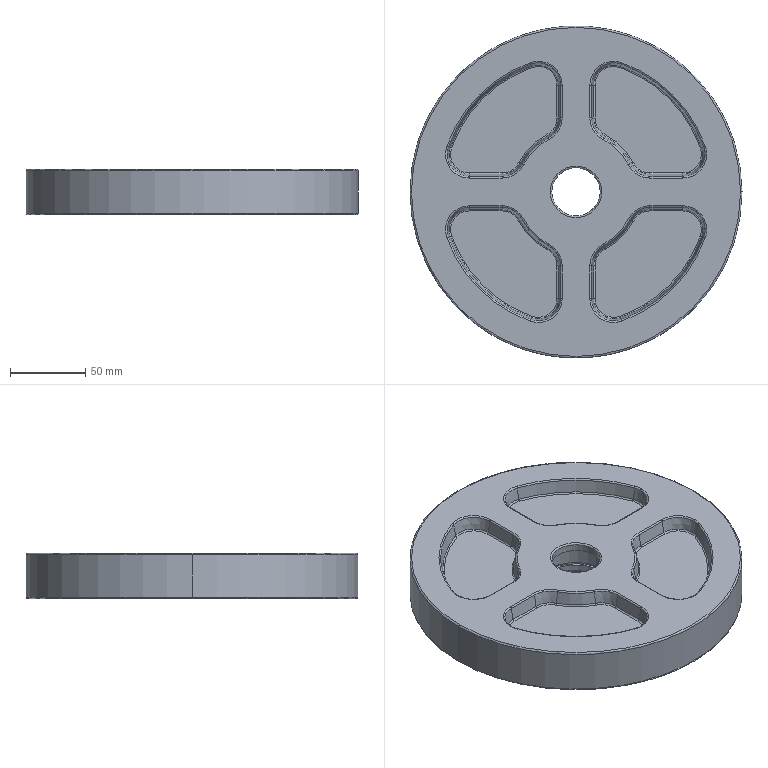Part | SolidWorks | features ICE 7, Fillet 2, CirPattern 1, Extrusion 1, MirrorPattern 1 | 1 solid | 243 faces | box 220 x 220 x 30 mm | volume 789072 mm3 | torus 112 | cylinder 50 | cone 48 | plane 33 | commonest cylinder face diameters 2 x32 3 x6 52 x4 32 x2 45 x2 55 x2